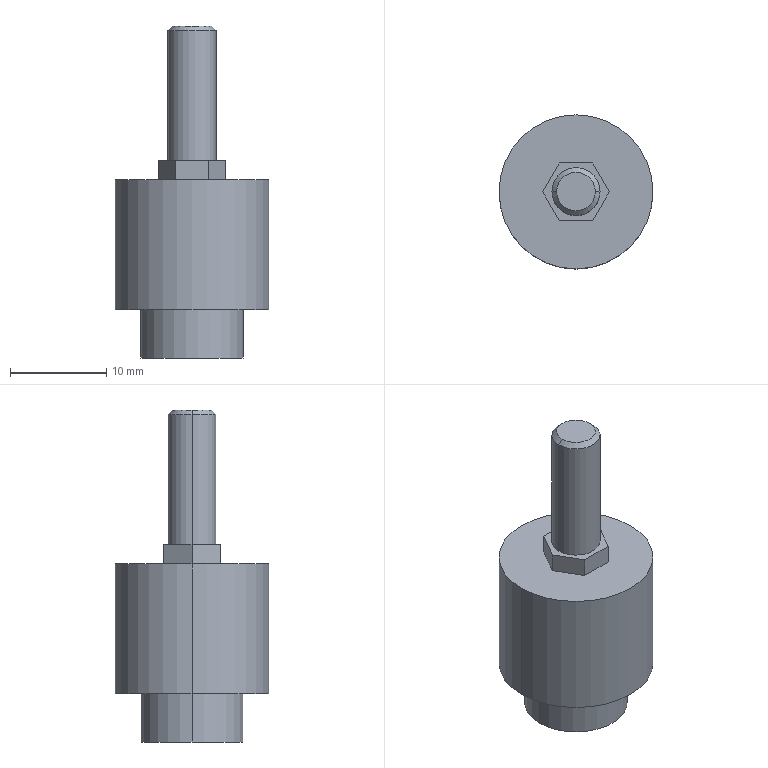Part | STEP file | JA15_5_080 | 1 solid | 24 faces | box 16 x 16 x 34.5 mm | volume 3402 mm3 | plane 12 | cylinder 8 | cone 4 | commonest cylinder face diameters 4.13 x2 5 x2 10.667 x2 16 x2
STEP:
#1=CARTESIAN_POINT('',(0.,0.,0.));
#2=DIRECTION('',(0.,0.,1.));
#3=DIRECTION('',(1.,0.,0.));
#4=AXIS2_PLACEMENT_3D('',#1,#2,#3);
#5=CARTESIAN_POINT('',(-2.5,0.,34.01));
#6=VERTEX_POINT('',#5);
#7=CARTESIAN_POINT('',(2.5,0.,34.01));
#8=VERTEX_POINT('',#7);
#9=CARTESIAN_POINT('',(0.,0.,34.01));
#10=DIRECTION('',(0.,0.,-1.));
#11=DIRECTION('',(-1.,0.,0.));
#12=AXIS2_PLACEMENT_3D('',#9,#10,#11);
#13=CIRCLE('',#12,2.5);
#14=CARTESIAN_POINT('',(0.,0.,20.5));
#15=DIRECTION('',(0.,0.,-1.));
#16=DIRECTION('',(-1.,0.,0.));
#17=AXIS2_PLACEMENT_3D('',#14,#15,#16);
#18=CYLINDRICAL_SURFACE('',#17,2.5);
#19=CARTESIAN_POINT('',(0.,-13.51));
#20=DIRECTION('',(1.,0.));
#21=VECTOR('',#20,1.);
#22=LINE('',#19,#21);
#23=(GEOMETRIC_REPRESENTATION_CONTEXT(2)PARAMETRIC_REPRESENTATION_CONTEXT()REPRESENTATION_CONTEXT('',''));
#24=DEFINITIONAL_REPRESENTATION('',(#22),#23);
#25=PCURVE('',#18,#24);
#26=CARTESIAN_POINT('',(0.,0.,34.01));
#27=DIRECTION('',(0.,0.,-1.));
#28=DIRECTION('',(-1.,0.,0.));
#29=AXIS2_PLACEMENT_3D('',#26,#27,#28);
#30=CONICAL_SURFACE('',#29,2.5,0.7854);
#31=CARTESIAN_POINT('',(0.,0.));
#32=DIRECTION('',(1.,0.));
#33=VECTOR('',#32,1.);
#34=LINE('',#31,#33);
#35=(GEOMETRIC_REPRESENTATION_CONTEXT(2)PARAMETRIC_REPRESENTATION_CONTEXT()REPRESENTATION_CONTEXT('',''));
#36=DEFINITIONAL_REPRESENTATION('',(#34),#35);
#37=PCURVE('',#30,#36);
#38=SURFACE_CURVE('',#13,(#25,#37),.PCURVE_S1.);
#39=EDGE_CURVE('',#6,#8,#38,.T.);
#40=ORIENTED_EDGE('',*,*,#39,.T.);
#41=CARTESIAN_POINT('',(2.5,0.,20.5));
#42=VERTEX_POINT('',#41);
#43=CARTESIAN_POINT('',(2.5,0.,20.5));
#44=DIRECTION('',(0.,0.,-1.));
#45=VECTOR('',#44,1.);
#46=LINE('',#43,#45);
#47=CARTESIAN_POINT('',(3.142,0.));
#48=DIRECTION('',(0.,1.));
#49=VECTOR('',#48,1.);
#50=LINE('',#47,#49);
#51=(GEOMETRIC_REPRESENTATION_CONTEXT(2)PARAMETRIC_REPRESENTATION_CONTEXT()REPRESENTATION_CONTEXT('',''));
#52=DEFINITIONAL_REPRESENTATION('',(#50),#51);
#53=PCURVE('',#18,#52);
#54=CARTESIAN_POINT('',(0.,0.,20.5));
#55=DIRECTION('',(0.,0.,-1.));
#56=DIRECTION('',(-1.,0.,0.));
#57=AXIS2_PLACEMENT_3D('',#54,#55,#56);
#58=CYLINDRICAL_SURFACE('',#57,2.5);
#59=CARTESIAN_POINT('',(3.142,0.));
#60=DIRECTION('',(0.,1.));
#61=VECTOR('',#60,1.);
#62=LINE('',#59,#61);
#63=(GEOMETRIC_REPRESENTATION_CONTEXT(2)PARAMETRIC_REPRESENTATION_CONTEXT()REPRESENTATION_CONTEXT('',''));
#64=DEFINITIONAL_REPRESENTATION('',(#62),#63);
#65=PCURVE('',#58,#64);
#66=SURFACE_CURVE('',#46,(#53,#65),.PCURVE_S1.);
#67=EDGE_CURVE('',#8,#42,#66,.T.);
#68=ORIENTED_EDGE('',*,*,#67,.T.);
#69=CARTESIAN_POINT('',(-2.5,0.,20.5));
#70=VERTEX_POINT('',#69);
#71=CARTESIAN_POINT('',(0.,0.,20.5));
#72=DIRECTION('',(0.,0.,1.));
#73=DIRECTION('',(1.,0.,0.));
#74=AXIS2_PLACEMENT_3D('',#71,#72,#73);
#75=CIRCLE('',#74,2.5);
#76=CARTESIAN_POINT('',(3.142,0.));
#77=DIRECTION('',(-1.,0.));
#78=VECTOR('',#77,1.);
#79=LINE('',#76,#78);
#80=(GEOMETRIC_REPRESENTATION_CONTEXT(2)PARAMETRIC_REPRESENTATION_CONTEXT()REPRESENTATION_CONTEXT('',''));
#81=DEFINITIONAL_REPRESENTATION('',(#79),#80);
#82=PCURVE('',#18,#81);
#83=CARTESIAN_POINT('',(-1.732,-3.,20.5));
#84=DIRECTION('',(0.,0.,1.));
#85=DIRECTION('',(1.,0.,0.));
#86=AXIS2_PLACEMENT_3D('',#83,#84,#85);
#87=PLANE('',#86);
#88=CARTESIAN_POINT('',(1.732,3.));
#89=DIRECTION('',(1.,0.));
#90=AXIS2_PLACEMENT_2D('',#88,#89);
#91=CIRCLE('',#90,2.5);
#92=(GEOMETRIC_REPRESENTATION_CONTEXT(2)PARAMETRIC_REPRESENTATION_CONTEXT()REPRESENTATION_CONTEXT('',''));
#93=DEFINITIONAL_REPRESENTATION('',(#91),#92);
#94=PCURVE('',#87,#93);
#95=SURFACE_CURVE('',#75,(#82,#94),.PCURVE_S1.);
#96=EDGE_CURVE('',#42,#70,#95,.T.);
#97=ORIENTED_EDGE('',*,*,#96,.T.);
#98=CARTESIAN_POINT('',(-2.5,0.,20.5));
#99=DIRECTION('',(0.,0.,-1.));
#100=VECTOR('',#99,1.);
#101=LINE('',#98,#100);
#102=CARTESIAN_POINT('',(0.,0.));
#103=DIRECTION('',(0.,1.));
#104=VECTOR('',#103,1.);
#105=LINE('',#102,#104);
#106=(GEOMETRIC_REPRESENTATION_CONTEXT(2)PARAMETRIC_REPRESENTATION_CONTEXT()REPRESENTATION_CONTEXT('',''));
#107=DEFINITIONAL_REPRESENTATION('',(#105),#106);
#108=PCURVE('',#18,#107);
#109=CARTESIAN_POINT('',(6.283,0.));
#110=DIRECTION('',(0.,1.));
#111=VECTOR('',#110,1.);
#112=LINE('',#109,#111);
#113=(GEOMETRIC_REPRESENTATION_CONTEXT(2)PARAMETRIC_REPRESENTATION_CONTEXT()REPRESENTATION_CONTEXT('',''));
#114=DEFINITIONAL_REPRESENTATION('',(#112),#113);
#115=PCURVE('',#58,#114);
#116=SURFACE_CURVE('',#101,(#108,#115),.PCURVE_S1.);
#117=EDGE_CURVE('',#6,#70,#116,.T.);
#118=ORIENTED_EDGE('',*,*,#117,.F.);
#119=EDGE_LOOP('',(#40,#68,#97,#118));
#120=FACE_BOUND('',#119,.T.);
#121=ADVANCED_FACE('',(#120),#18,.T.);
#122=CARTESIAN_POINT('',(-2.01,0.,34.5));
#123=VERTEX_POINT('',#122);
#124=CARTESIAN_POINT('',(2.01,0.,34.5));
#125=VERTEX_POINT('',#124);
#126=CARTESIAN_POINT('',(0.,0.,34.5));
#127=DIRECTION('',(0.,0.,-1.));
#128=DIRECTION('',(-1.,0.,0.));
#129=AXIS2_PLACEMENT_3D('',#126,#127,#128);
#130=CIRCLE('',#129,2.01);
#131=CARTESIAN_POINT('',(0.,-0.49));
#132=DIRECTION('',(1.,0.));
#133=VECTOR('',#132,1.);
#134=LINE('',#131,#133);
#135=(GEOMETRIC_REPRESENTATION_CONTEXT(2)PARAMETRIC_REPRESENTATION_CONTEXT()REPRESENTATION_CONTEXT('',''));
#136=DEFINITIONAL_REPRESENTATION('',(#134),#135);
#137=PCURVE('',#30,#136);
#138=CARTESIAN_POINT('',(0.,0.,34.5));
#139=DIRECTION('',(0.,0.,1.));
#140=DIRECTION('',(1.,0.,0.));
#141=AXIS2_PLACEMENT_3D('',#138,#139,#140);
#142=PLANE('',#141);
#143=CARTESIAN_POINT('',(-2.01,0.));
#144=CARTESIAN_POINT('',(-2.01,3.481));
#145=CARTESIAN_POINT('',(1.005,1.741));
#146=CARTESIAN_POINT('',(4.02,0.));
#147=CARTESIAN_POINT('',(1.005,-1.741));
#148=CARTESIAN_POINT('',(-2.01,-3.481));
#149=CARTESIAN_POINT('',(-2.01,0.));
#150=(BOUNDED_CURVE()B_SPLINE_CURVE(2,(#143,#144,#145,#146,#147,#148,#149),.UNSPECIFIED.,.T.,.F.)B_SPLINE_CURVE_WITH_KNOTS((1,2,2,2,2,1),(-2.094,0.,2.094,4.189,6.283,8.378),.UNSPECIFIED.)CURVE()GEOMETRIC_REPRESENTATION_ITEM()RATIONAL_B_SPLINE_CURVE((1.,0.5,1.,0.5,1.,0.5,1.))REPRESENTATION_ITEM(''));
#151=(GEOMETRIC_REPRESENTATION_CONTEXT(2)PARAMETRIC_REPRESENTATION_CONTEXT()REPRESENTATION_CONTEXT('',''));
#152=DEFINITIONAL_REPRESENTATION('',(#150),#151);
#153=PCURVE('',#142,#152);
#154=SURFACE_CURVE('',#130,(#137,#153),.PCURVE_S1.);
#155=EDGE_CURVE('',#123,#125,#154,.T.);
#156=ORIENTED_EDGE('',*,*,#155,.T.);
#157=CARTESIAN_POINT('',(2.5,0.,34.01));
#158=DIRECTION('',(0.7071,0.,-0.7071));
#159=VECTOR('',#158,1.);
#160=LINE('',#157,#159);
#161=CARTESIAN_POINT('',(3.142,0.));
#162=DIRECTION('',(0.,1.));
#163=VECTOR('',#162,1.);
#164=LINE('',#161,#163);
#165=(GEOMETRIC_REPRESENTATION_CONTEXT(2)PARAMETRIC_REPRESENTATION_CONTEXT()REPRESENTATION_CONTEXT('',''));
#166=DEFINITIONAL_REPRESENTATION('',(#164),#165);
#167=PCURVE('',#30,#166);
#168=CARTESIAN_POINT('',(0.,0.,34.01));
#169=DIRECTION('',(0.,0.,-1.));
#170=DIRECTION('',(-1.,0.,0.));
#171=AXIS2_PLACEMENT_3D('',#168,#169,#170);
#172=CONICAL_SURFACE('',#171,2.5,0.7854);
#173=CARTESIAN_POINT('',(3.142,0.));
#174=DIRECTION('',(0.,1.));
#175=VECTOR('',#174,1.);
#176=LINE('',#173,#175);
#177=(GEOMETRIC_REPRESENTATION_CONTEXT(2)PARAMETRIC_REPRESENTATION_CONTEXT()REPRESENTATION_CONTEXT('',''));
#178=DEFINITIONAL_REPRESENTATION('',(#176),#177);
#179=PCURVE('',#172,#178);
#180=SURFACE_CURVE('',#160,(#167,#179),.PCURVE_S1.);
#181=EDGE_CURVE('',#125,#8,#180,.T.);
#182=ORIENTED_EDGE('',*,*,#181,.T.);
#183=ORIENTED_EDGE('',*,*,#39,.F.);
#184=CARTESIAN_POINT('',(-2.5,0.,34.01));
#185=DIRECTION('',(-0.7071,0.,-0.7071));
#186=VECTOR('',#185,1.);
#187=LINE('',#184,#186);
#188=CARTESIAN_POINT('',(0.,0.));
#189=DIRECTION('',(0.,1.));
#190=VECTOR('',#189,1.);
#191=LINE('',#188,#190);
#192=(GEOMETRIC_REPRESENTATION_CONTEXT(2)PARAMETRIC_REPRESENTATION_CONTEXT()REPRESENTATION_CONTEXT('',''));
#193=DEFINITIONAL_REPRESENTATION('',(#191),#192);
#194=PCURVE('',#30,#193);
#195=CARTESIAN_POINT('',(6.283,0.));
#196=DIRECTION('',(0.,1.));
#197=VECTOR('',#196,1.);
#198=LINE('',#195,#197);
#199=(GEOMETRIC_REPRESENTATION_CONTEXT(2)PARAMETRIC_REPRESENTATION_CONTEXT()REPRESENTATION_CONTEXT('',''));
#200=DEFINITIONAL_REPRESENTATION('',(#198),#199);
#201=PCURVE('',#172,#200);
#202=SURFACE_CURVE('',#187,(#194,#201),.PCURVE_S1.);
#203=EDGE_CURVE('',#123,#6,#202,.T.);
#204=ORIENTED_EDGE('',*,*,#203,.F.);
#205=EDGE_LOOP('',(#156,#182,#183,#204));
#206=FACE_BOUND('',#205,.T.);
#207=ADVANCED_FACE('',(#206),#30,.T.);
#208=CARTESIAN_POINT('',(-2.065,0.,7.));
#209=VERTEX_POINT('',#208);
#210=CARTESIAN_POINT('',(-2.065,0.,0.435));
#211=VERTEX_POINT('',#210);
#212=CARTESIAN_POINT('',(-2.065,0.,0.));
#213=DIRECTION('',(0.,0.,-1.));
#214=VECTOR('',#213,1.);
#215=LINE('',#212,#214);
#216=CARTESIAN_POINT('',(0.,0.,0.));
#217=DIRECTION('',(0.,0.,-1.));
#218=DIRECTION('',(-1.,0.,0.));
#219=AXIS2_PLACEMENT_3D('',#216,#217,#218);
#220=CYLINDRICAL_SURFACE('',#219,2.065);
#221=CARTESIAN_POINT('',(6.283,0.));
#222=DIRECTION('',(0.,1.));
#223=VECTOR('',#222,1.);
#224=LINE('',#221,#223);
#225=(GEOMETRIC_REPRESENTATION_CONTEXT(2)PARAMETRIC_REPRESENTATION_CONTEXT()REPRESENTATION_CONTEXT('',''));
#226=DEFINITIONAL_REPRESENTATION('',(#224),#225);
#227=PCURVE('',#220,#226);
#228=CARTESIAN_POINT('',(0.,0.,0.));
#229=DIRECTION('',(0.,0.,-1.));
#230=DIRECTION('',(-1.,0.,0.));
#231=AXIS2_PLACEMENT_3D('',#228,#229,#230);
#232=CYLINDRICAL_SURFACE('',#231,2.065);
#233=CARTESIAN_POINT('',(0.,0.));
#234=DIRECTION('',(0.,1.));
#235=VECTOR('',#234,1.);
#236=LINE('',#233,#235);
#237=(GEOMETRIC_REPRESENTATION_CONTEXT(2)PARAMETRIC_REPRESENTATION_CONTEXT()REPRESENTATION_CONTEXT('',''));
#238=DEFINITIONAL_REPRESENTATION('',(#236),#237);
#239=PCURVE('',#232,#238);
#240=SURFACE_CURVE('',#215,(#227,#239),.PCURVE_S1.);
#241=EDGE_CURVE('',#209,#211,#240,.T.);
#242=ORIENTED_EDGE('',*,*,#241,.T.);
#243=CARTESIAN_POINT('',(2.065,0.,0.435));
#244=VERTEX_POINT('',#243);
#245=CARTESIAN_POINT('',(0.,0.,0.435));
#246=DIRECTION('',(0.,0.,-1.));
#247=DIRECTION('',(-1.,0.,0.));
#248=AXIS2_PLACEMENT_3D('',#245,#246,#247);
#249=CIRCLE('',#248,2.065);
#250=CARTESIAN_POINT('',(0.,-0.435));
#251=DIRECTION('',(1.,0.));
#252=VECTOR('',#251,1.);
#253=LINE('',#250,#252);
#254=(GEOMETRIC_REPRESENTATION_CONTEXT(2)PARAMETRIC_REPRESENTATION_CONTEXT()REPRESENTATION_CONTEXT('',''));
#255=DEFINITIONAL_REPRESENTATION('',(#253),#254);
#256=PCURVE('',#220,#255);
#257=CARTESIAN_POINT('',(0.,0.,0.435));
#258=DIRECTION('',(0.,0.,-1.));
#259=DIRECTION('',(-1.,0.,0.));
#260=AXIS2_PLACEMENT_3D('',#257,#258,#259);
#261=CONICAL_SURFACE('',#260,2.065,0.7854);
#262=CARTESIAN_POINT('',(0.,0.));
#263=DIRECTION('',(1.,0.));
#264=VECTOR('',#263,1.);
#265=LINE('',#262,#264);
#266=(GEOMETRIC_REPRESENTATION_CONTEXT(2)PARAMETRIC_REPRESENTATION_CONTEXT()REPRESENTATION_CONTEXT('',''));
#267=DEFINITIONAL_REPRESENTATION('',(#265),#266);
#268=PCURVE('',#261,#267);
#269=SURFACE_CURVE('',#249,(#256,#268),.PCURVE_S1.);
#270=EDGE_CURVE('',#244,#211,#269,.T.);
#271=ORIENTED_EDGE('',*,*,#270,.F.);
#272=CARTESIAN_POINT('',(2.065,0.,7.));
#273=VERTEX_POINT('',#272);
#274=CARTESIAN_POINT('',(2.065,0.,0.));
#275=DIRECTION('',(0.,0.,-1.));
#276=VECTOR('',#275,1.);
#277=LINE('',#274,#276);
#278=CARTESIAN_POINT('',(3.142,0.));
#279=DIRECTION('',(0.,1.));
#280=VECTOR('',#279,1.);
#281=LINE('',#278,#280);
#282=(GEOMETRIC_REPRESENTATION_CONTEXT(2)PARAMETRIC_REPRESENTATION_CONTEXT()REPRESENTATION_CONTEXT('',''));
#283=DEFINITIONAL_REPRESENTATION('',(#281),#282);
#284=PCURVE('',#220,#283);
#285=CARTESIAN_POINT('',(3.142,0.));
#286=DIRECTION('',(0.,1.));
#287=VECTOR('',#286,1.);
#288=LINE('',#285,#287);
#289=(GEOMETRIC_REPRESENTATION_CONTEXT(2)PARAMETRIC_REPRESENTATION_CONTEXT()REPRESENTATION_CONTEXT('',''));
#290=DEFINITIONAL_REPRESENTATION('',(#288),#289);
#291=PCURVE('',#232,#290);
#292=SURFACE_CURVE('',#277,(#284,#291),.PCURVE_S1.);
#293=EDGE_CURVE('',#273,#244,#292,.T.);
#294=ORIENTED_EDGE('',*,*,#293,.F.);
#295=CARTESIAN_POINT('',(0.,0.,7.));
#296=DIRECTION('',(0.,0.,-1.));
#297=DIRECTION('',(-1.,0.,0.));
#298=AXIS2_PLACEMENT_3D('',#295,#296,#297);
#299=CIRCLE('',#298,2.065);
#300=CARTESIAN_POINT('',(0.,-7.));
#301=DIRECTION('',(1.,0.));
#302=VECTOR('',#301,1.);
#303=LINE('',#300,#302);
#304=(GEOMETRIC_REPRESENTATION_CONTEXT(2)PARAMETRIC_REPRESENTATION_CONTEXT()REPRESENTATION_CONTEXT('',''));
#305=DEFINITIONAL_REPRESENTATION('',(#303),#304);
#306=PCURVE('',#220,#305);
#307=CARTESIAN_POINT('',(0.,2.065,7.));
#308=DIRECTION('',(0.,0.,-1.));
#309=DIRECTION('',(-1.,0.,0.));
#310=AXIS2_PLACEMENT_3D('',#307,#308,#309);
#311=PLANE('',#310);
#312=CARTESIAN_POINT('',(0.,-2.065));
#313=DIRECTION('',(1.,0.));
#314=AXIS2_PLACEMENT_2D('',#312,#313);
#315=CIRCLE('',#314,2.065);
#316=(GEOMETRIC_REPRESENTATION_CONTEXT(2)PARAMETRIC_REPRESENTATION_CONTEXT()REPRESENTATION_CONTEXT('',''));
#317=DEFINITIONAL_REPRESENTATION('',(#315),#316);
#318=PCURVE('',#311,#317);
#319=SURFACE_CURVE('',#299,(#306,#318),.PCURVE_S1.);
#320=EDGE_CURVE('',#273,#209,#319,.T.);
#321=ORIENTED_EDGE('',*,*,#320,.T.);
#322=EDGE_LOOP('',(#242,#271,#294,#321));
#323=FACE_BOUND('',#322,.F.);
#324=ADVANCED_FACE('',(#323),#220,.F.);
#325=CARTESIAN_POINT('',(-2.5,0.,0.));
#326=VERTEX_POINT('',#325);
#327=CARTESIAN_POINT('',(-2.065,0.,0.435));
#328=DIRECTION('',(-0.7071,0.,-0.7071));
#329=VECTOR('',#328,1.);
#330=LINE('',#327,#329);
#331=CARTESIAN_POINT('',(6.283,0.));
#332=DIRECTION('',(0.,1.));
#333=VECTOR('',#332,1.);
#334=LINE('',#331,#333);
#335=(GEOMETRIC_REPRESENTATION_CONTEXT(2)PARAMETRIC_REPRESENTATION_CONTEXT()REPRESENTATION_CONTEXT('',''));
#336=DEFINITIONAL_REPRESENTATION('',(#334),#335);
#337=PCURVE('',#261,#336);
#338=CARTESIAN_POINT('',(0.,0.,0.435));
#339=DIRECTION('',(0.,0.,-1.));
#340=DIRECTION('',(-1.,0.,0.));
#341=AXIS2_PLACEMENT_3D('',#338,#339,#340);
#342=CONICAL_SURFACE('',#341,2.065,0.7854);
#343=CARTESIAN_POINT('',(0.,0.));
#344=DIRECTION('',(0.,1.));
#345=VECTOR('',#344,1.);
#346=LINE('',#343,#345);
#347=(GEOMETRIC_REPRESENTATION_CONTEXT(2)PARAMETRIC_REPRESENTATION_CONTEXT()REPRESENTATION_CONTEXT('',''));
#348=DEFINITIONAL_REPRESENTATION('',(#346),#347);
#349=PCURVE('',#342,#348);
#350=SURFACE_CURVE('',#330,(#337,#349),.PCURVE_S1.);
#351=EDGE_CURVE('',#211,#326,#350,.T.);
#352=ORIENTED_EDGE('',*,*,#351,.T.);
#353=CARTESIAN_POINT('',(2.5,0.,0.));
#354=VERTEX_POINT('',#353);
#355=CARTESIAN_POINT('',(0.,0.,0.));
#356=DIRECTION('',(0.,0.,-1.));
#357=DIRECTION('',(-1.,0.,0.));
#358=AXIS2_PLACEMENT_3D('',#355,#356,#357);
#359=CIRCLE('',#358,2.5);
#360=CARTESIAN_POINT('',(0.,0.435));
#361=DIRECTION('',(1.,0.));
#362=VECTOR('',#361,1.);
#363=LINE('',#360,#362);
#364=(GEOMETRIC_REPRESENTATION_CONTEXT(2)PARAMETRIC_REPRESENTATION_CONTEXT()REPRESENTATION_CONTEXT('',''));
#365=DEFINITIONAL_REPRESENTATION('',(#363),#364);
#366=PCURVE('',#261,#365);
#367=CARTESIAN_POINT('',(0.,5.333,0.));
#368=DIRECTION('',(0.,0.,-1.));
#369=DIRECTION('',(-1.,0.,0.));
#370=AXIS2_PLACEMENT_3D('',#367,#368,#369);
#371=PLANE('',#370);
#372=CARTESIAN_POINT('',(0.,-5.333));
#373=DIRECTION('',(1.,0.));
#374=AXIS2_PLACEMENT_2D('',#372,#373);
#375=CIRCLE('',#374,2.5);
#376=(GEOMETRIC_REPRESENTATION_CONTEXT(2)PARAMETRIC_REPRESENTATION_CONTEXT()REPRESENTATION_CONTEXT('',''));
#377=DEFINITIONAL_REPRESENTATION('',(#375),#376);
#378=PCURVE('',#371,#377);
#379=SURFACE_CURVE('',#359,(#366,#378),.PCURVE_S1.);
#380=EDGE_CURVE('',#354,#326,#379,.T.);
#381=ORIENTED_EDGE('',*,*,#380,.F.);
#382=CARTESIAN_POINT('',(2.065,0.,0.435));
#383=DIRECTION('',(0.7071,0.,-0.7071));
#384=VECTOR('',#383,1.);
#385=LINE('',#382,#384);
#386=CARTESIAN_POINT('',(3.142,0.));
#387=DIRECTION('',(0.,1.));
#388=VECTOR('',#387,1.);
#389=LINE('',#386,#388);
#390=(GEOMETRIC_REPRESENTATION_CONTEXT(2)PARAMETRIC_REPRESENTATION_CONTEXT()REPRESENTATION_CONTEXT('',''));
#391=DEFINITIONAL_REPRESENTATION('',(#389),#390);
#392=PCURVE('',#261,#391);
#393=CARTESIAN_POINT('',(3.142,0.));
#394=DIRECTION('',(0.,1.));
#395=VECTOR('',#394,1.);
#396=LINE('',#393,#395);
#397=(GEOMETRIC_REPRESENTATION_CONTEXT(2)PARAMETRIC_REPRESENTATION_CONTEXT()REPRESENTATION_CONTEXT('',''));
#398=DEFINITIONAL_REPRESENTATION('',(#396),#397);
#399=PCURVE('',#342,#398);
#400=SURFACE_CURVE('',#385,(#392,#399),.PCURVE_S1.);
#401=EDGE_CURVE('',#244,#354,#400,.T.);
#402=ORIENTED_EDGE('',*,*,#401,.F.);
#403=ORIENTED_EDGE('',*,*,#270,.T.);
#404=EDGE_LOOP('',(#352,#381,#402,#403));
#405=FACE_BOUND('',#404,.F.);
#406=ADVANCED_FACE('',(#405),#261,.F.);
#407=CARTESIAN_POINT('',(-5.333,0.,5.));
#408=VERTEX_POINT('',#407);
#409=CARTESIAN_POINT('',(5.333,0.,5.));
#410=VERTEX_POINT('',#409);
#411=CARTESIAN_POINT('',(0.,0.,5.));
#412=DIRECTION('',(0.,0.,-1.));
#413=DIRECTION('',(-1.,0.,0.));
#414=AXIS2_PLACEMENT_3D('',#411,#412,#413);
#415=CIRCLE('',#414,5.333);
#416=CARTESIAN_POINT('',(0.,0.,0.));
#417=DIRECTION('',(0.,0.,-1.));
#418=DIRECTION('',(-1.,0.,0.));
#419=AXIS2_PLACEMENT_3D('',#416,#417,#418);
#420=CYLINDRICAL_SURFACE('',#419,5.333);
#421=CARTESIAN_POINT('',(0.,-5.));
#422=DIRECTION('',(1.,0.));
#423=VECTOR('',#422,1.);
#424=LINE('',#421,#423);
#425=(GEOMETRIC_REPRESENTATION_CONTEXT(2)PARAMETRIC_REPRESENTATION_CONTEXT()REPRESENTATION_CONTEXT('',''));
#426=DEFINITIONAL_REPRESENTATION('',(#424),#425);
#427=PCURVE('',#420,#426);
#428=CARTESIAN_POINT('',(0.,8.,5.));
#429=DIRECTION('',(0.,0.,-1.));
#430=DIRECTION('',(-1.,0.,0.));
#431=AXIS2_PLACEMENT_3D('',#428,#429,#430);
#432=PLANE('',#431);
#433=CARTESIAN_POINT('',(0.,-8.));
#434=DIRECTION('',(1.,0.));
#435=AXIS2_PLACEMENT_2D('',#433,#434);
#436=CIRCLE('',#435,5.333);
#437=(GEOMETRIC_REPRESENTATION_CONTEXT(2)PARAMETRIC_REPRESENTATION_CONTEXT()REPRESENTATION_CONTEXT('',''));
#438=DEFINITIONAL_REPRESENTATION('',(#436),#437);
#439=PCURVE('',#432,#438);
#440=SURFACE_CURVE('',#415,(#427,#439),.PCURVE_S1.);
#441=EDGE_CURVE('',#408,#410,#440,.T.);
#442=ORIENTED_EDGE('',*,*,#441,.T.);
#443=CARTESIAN_POINT('',(5.333,0.,0.));
#444=VERTEX_POINT('',#443);
#445=CARTESIAN_POINT('',(5.333,0.,0.));
#446=DIRECTION('',(0.,0.,-1.));
#447=VECTOR('',#446,1.);
#448=LINE('',#445,#447);
#449=CARTESIAN_POINT('',(3.142,0.));
#450=DIRECTION('',(0.,1.));
#451=VECTOR('',#450,1.);
#452=LINE('',#449,#451);
#453=(GEOMETRIC_REPRESENTATION_CONTEXT(2)PARAMETRIC_REPRESENTATION_CONTEXT()REPRESENTATION_CONTEXT('',''));
#454=DEFINITIONAL_REPRESENTATION('',(#452),#453);
#455=PCURVE('',#420,#454);
#456=CARTESIAN_POINT('',(0.,0.,0.));
#457=DIRECTION('',(0.,0.,-1.));
#458=DIRECTION('',(-1.,0.,0.));
#459=AXIS2_PLACEMENT_3D('',#456,#457,#458);
#460=CYLINDRICAL_SURFACE('',#459,5.333);
#461=CARTESIAN_POINT('',(3.142,0.));
#462=DIRECTION('',(0.,1.));
#463=VECTOR('',#462,1.);
#464=LINE('',#461,#463);
#465=(GEOMETRIC_REPRESENTATION_CONTEXT(2)PARAMETRIC_REPRESENTATION_CONTEXT()REPRESENTATION_CONTEXT('',''));
#466=DEFINITIONAL_REPRESENTATION('',(#464),#465);
#467=PCURVE('',#460,#466);
#468=SURFACE_CURVE('',#448,(#455,#467),.PCURVE_S1.);
#469=EDGE_CURVE('',#410,#444,#468,.T.);
#470=ORIENTED_EDGE('',*,*,#469,.T.);
#471=CARTESIAN_POINT('',(-5.333,0.,0.));
#472=VERTEX_POINT('',#471);
#473=CARTESIAN_POINT('',(0.,0.,0.));
#474=DIRECTION('',(0.,0.,-1.));
#475=DIRECTION('',(-1.,0.,0.));
#476=AXIS2_PLACEMENT_3D('',#473,#474,#475);
#477=CIRCLE('',#476,5.333);
#478=CARTESIAN_POINT('',(0.,0.));
#479=DIRECTION('',(1.,0.));
#480=VECTOR('',#479,1.);
#481=LINE('',#478,#480);
#482=(GEOMETRIC_REPRESENTATION_CONTEXT(2)PARAMETRIC_REPRESENTATION_CONTEXT()REPRESENTATION_CONTEXT('',''));
#483=DEFINITIONAL_REPRESENTATION('',(#481),#482);
#484=PCURVE('',#420,#483);
#485=CARTESIAN_POINT('',(0.,-5.333));
#486=DIRECTION('',(1.,0.));
#487=AXIS2_PLACEMENT_2D('',#485,#486);
#488=CIRCLE('',#487,5.333);
#489=(GEOMETRIC_REPRESENTATION_CONTEXT(2)PARAMETRIC_REPRESENTATION_CONTEXT()REPRESENTATION_CONTEXT('',''));
#490=DEFINITIONAL_REPRESENTATION('',(#488),#489);
#491=PCURVE('',#371,#490);
#492=SURFACE_CURVE('',#477,(#484,#491),.PCURVE_S1.);
#493=EDGE_CURVE('',#472,#444,#492,.T.);
#494=ORIENTED_EDGE('',*,*,#493,.F.);
#495=CARTESIAN_POINT('',(-5.333,0.,0.));
#496=DIRECTION('',(0.,0.,-1.));
#497=VECTOR('',#496,1.);
#498=LINE('',#495,#497);
#499=CARTESIAN_POINT('',(0.,0.));
#500=DIRECTION('',(0.,1.));
#501=VECTOR('',#500,1.);
#502=LINE('',#499,#501);
#503=(GEOMETRIC_REPRESENTATION_CONTEXT(2)PARAMETRIC_REPRESENTATION_CONTEXT()REPRESENTATION_CONTEXT('',''));
#504=DEFINITIONAL_REPRESENTATION('',(#502),#503);
#505=PCURVE('',#420,#504);
#506=CARTESIAN_POINT('',(6.283,0.));
#507=DIRECTION('',(0.,1.));
#508=VECTOR('',#507,1.);
#509=LINE('',#506,#508);
#510=(GEOMETRIC_REPRESENTATION_CONTEXT(2)PARAMETRIC_REPRESENTATION_CONTEXT()REPRESENTATION_CONTEXT('',''));
#511=DEFINITIONAL_REPRESENTATION('',(#509),#510);
#512=PCURVE('',#460,#511);
#513=SURFACE_CURVE('',#498,(#505,#512),.PCURVE_S1.);
#514=EDGE_CURVE('',#408,#472,#513,.T.);
#515=ORIENTED_EDGE('',*,*,#514,.F.);
#516=EDGE_LOOP('',(#442,#470,#494,#515));
#517=FACE_BOUND('',#516,.T.);
#518=ADVANCED_FACE('',(#517),#420,.T.);
#519=CARTESIAN_POINT('',(-8.,0.,18.5));
#520=VERTEX_POINT('',#519);
#521=CARTESIAN_POINT('',(8.,0.,18.5));
#522=VERTEX_POINT('',#521);
#523=CARTESIAN_POINT('',(0.,0.,18.5));
#524=DIRECTION('',(0.,0.,-1.));
#525=DIRECTION('',(-1.,0.,0.));
#526=AXIS2_PLACEMENT_3D('',#523,#524,#525);
#527=CIRCLE('',#526,8.);
#528=CARTESIAN_POINT('',(0.,0.,0.));
#529=DIRECTION('',(0.,0.,-1.));
#530=DIRECTION('',(-1.,0.,0.));
#531=AXIS2_PLACEMENT_3D('',#528,#529,#530);
#532=CYLINDRICAL_SURFACE('',#531,8.);
#533=CARTESIAN_POINT('',(0.,-18.5));
#534=DIRECTION('',(1.,0.));
#535=VECTOR('',#534,1.);
#536=LINE('',#533,#535);
#537=(GEOMETRIC_REPRESENTATION_CONTEXT(2)PARAMETRIC_REPRESENTATION_CONTEXT()REPRESENTATION_CONTEXT('',''));
#538=DEFINITIONAL_REPRESENTATION('',(#536),#537);
#539=PCURVE('',#532,#538);
#540=CARTESIAN_POINT('',(0.,0.,18.5));
#541=DIRECTION('',(0.,0.,1.));
#542=DIRECTION('',(1.,0.,0.));
#543=AXIS2_PLACEMENT_3D('',#540,#541,#542);
#544=PLANE('',#543);
#545=CARTESIAN_POINT('',(-8.,0.));
#546=CARTESIAN_POINT('',(-8.,13.856));
#547=CARTESIAN_POINT('',(4.,6.928));
#548=CARTESIAN_POINT('',(16.,0.));
#549=CARTESIAN_POINT('',(4.,-6.928));
#550=CARTESIAN_POINT('',(-8.,-13.856));
#551=CARTESIAN_POINT('',(-8.,0.));
#552=(BOUNDED_CURVE()B_SPLINE_CURVE(2,(#545,#546,#547,#548,#549,#550,#551),.UNSPECIFIED.,.T.,.F.)B_SPLINE_CURVE_WITH_KNOTS((1,2,2,2,2,1),(-2.094,0.,2.094,4.189,6.283,8.378),.UNSPECIFIED.)CURVE()GEOMETRIC_REPRESENTATION_ITEM()RATIONAL_B_SPLINE_CURVE((1.,0.5,1.,0.5,1.,0.5,1.))REPRESENTATION_ITEM(''));
#553=(GEOMETRIC_REPRESENTATION_CONTEXT(2)PARAMETRIC_REPRESENTATION_CONTEXT()REPRESENTATION_CONTEXT('',''));
#554=DEFINITIONAL_REPRESENTATION('',(#552),#553);
#555=PCURVE('',#544,#554);
#556=SURFACE_CURVE('',#527,(#539,#555),.PCURVE_S1.);
#557=EDGE_CURVE('',#520,#522,#556,.T.);
#558=ORIENTED_EDGE('',*,*,#557,.T.);
#559=CARTESIAN_POINT('',(8.,0.,5.));
#560=VERTEX_POINT('',#559);
#561=CARTESIAN_POINT('',(8.,0.,0.));
#562=DIRECTION('',(0.,0.,-1.));
#563=VECTOR('',#562,1.);
#564=LINE('',#561,#563);
#565=CARTESIAN_POINT('',(3.142,0.));
#566=DIRECTION('',(0.,1.));
#567=VECTOR('',#566,1.);
#568=LINE('',#565,#567);
#569=(GEOMETRIC_REPRESENTATION_CONTEXT(2)PARAMETRIC_REPRESENTATION_CONTEXT()REPRESENTATION_CONTEXT('',''));
#570=DEFINITIONAL_REPRESENTATION('',(#568),#569);
#571=PCURVE('',#532,#570);
#572=CARTESIAN_POINT('',(0.,0.,0.));
#573=DIRECTION('',(0.,0.,-1.));
#574=DIRECTION('',(-1.,0.,0.));
#575=AXIS2_PLACEMENT_3D('',#572,#573,#574);
#576=CYLINDRICAL_SURFACE('',#575,8.);
#577=CARTESIAN_POINT('',(3.142,0.));
#578=DIRECTION('',(0.,1.));
#579=VECTOR('',#578,1.);
#580=LINE('',#577,#579);
#581=(GEOMETRIC_REPRESENTATION_CONTEXT(2)PARAMETRIC_REPRESENTATION_CONTEXT()REPRESENTATION_CONTEXT('',''));
#582=DEFINITIONAL_REPRESENTATION('',(#580),#581);
#583=PCURVE('',#576,#582);
#584=SURFACE_CURVE('',#564,(#571,#583),.PCURVE_S1.);
#585=EDGE_CURVE('',#522,#560,#584,.T.);
#586=ORIENTED_EDGE('',*,*,#585,.T.);
#587=CARTESIAN_POINT('',(-8.,0.,5.));
#588=VERTEX_POINT('',#587);
#589=CARTESIAN_POINT('',(0.,0.,5.));
#590=DIRECTION('',(0.,0.,-1.));
#591=DIRECTION('',(-1.,0.,0.));
#592=AXIS2_PLACEMENT_3D('',#589,#590,#591);
#593=CIRCLE('',#592,8.);
#594=CARTESIAN_POINT('',(0.,-5.));
#595=DIRECTION('',(1.,0.));
#596=VECTOR('',#595,1.);
#597=LINE('',#594,#596);
#598=(GEOMETRIC_REPRESENTATION_CONTEXT(2)PARAMETRIC_REPRESENTATION_CONTEXT()REPRESENTATION_CONTEXT('',''));
#599=DEFINITIONAL_REPRESENTATION('',(#597),#598);
#600=PCURVE('',#532,#599);
#601=CARTESIAN_POINT('',(0.,-8.));
#602=DIRECTION('',(1.,0.));
#603=AXIS2_PLACEMENT_2D('',#601,#602);
#604=CIRCLE('',#603,8.);
#605=(GEOMETRIC_REPRESENTATION_CONTEXT(2)PARAMETRIC_REPRESENTATION_CONTEXT()REPRESENTATION_CONTEXT('',''));
#606=DEFINITIONAL_REPRESENTATION('',(#604),#605);
#607=PCURVE('',#432,#606);
#608=SURFACE_CURVE('',#593,(#600,#607),.PCURVE_S1.);
#609=EDGE_CURVE('',#588,#560,#608,.T.);
#610=ORIENTED_EDGE('',*,*,#609,.F.);
#611=CARTESIAN_POINT('',(-8.,0.,0.));
#612=DIRECTION('',(0.,0.,-1.));
#613=VECTOR('',#612,1.);
#614=LINE('',#611,#613);
#615=CARTESIAN_POINT('',(0.,0.));
#616=DIRECTION('',(0.,1.));
#617=VECTOR('',#616,1.);
#618=LINE('',#615,#617);
#619=(GEOMETRIC_REPRESENTATION_CONTEXT(2)PARAMETRIC_REPRESENTATION_CONTEXT()REPRESENTATION_CONTEXT('',''));
#620=DEFINITIONAL_REPRESENTATION('',(#618),#619);
#621=PCURVE('',#532,#620);
#622=CARTESIAN_POINT('',(6.283,0.));
#623=DIRECTION('',(0.,1.));
#624=VECTOR('',#623,1.);
#625=LINE('',#622,#624);
#626=(GEOMETRIC_REPRESENTATION_CONTEXT(2)PARAMETRIC_REPRESENTATION_CONTEXT()REPRESENTATION_CONTEXT('',''));
#627=DEFINITIONAL_REPRESENTATION('',(#625),#626);
#628=PCURVE('',#576,#627);
#629=SURFACE_CURVE('',#614,(#621,#628),.PCURVE_S1.);
#630=EDGE_CURVE('',#520,#588,#629,.T.);
#631=ORIENTED_EDGE('',*,*,#630,.F.);
#632=EDGE_LOOP('',(#558,#586,#610,#631));
#633=FACE_BOUND('',#632,.T.);
#634=ADVANCED_FACE('',(#633),#532,.T.);
#635=ORIENTED_EDGE('',*,*,#557,.F.);
#636=CARTESIAN_POINT('',(0.,0.,18.5));
#637=DIRECTION('',(0.,0.,-1.));
#638=DIRECTION('',(-1.,0.,0.));
#639=AXIS2_PLACEMENT_3D('',#636,#637,#638);
#640=CIRCLE('',#639,8.);
#641=CARTESIAN_POINT('',(-8.,0.));
#642=CARTESIAN_POINT('',(-8.,13.856));
#643=CARTESIAN_POINT('',(4.,6.928));
#644=CARTESIAN_POINT('',(16.,0.));
#645=CARTESIAN_POINT('',(4.,-6.928));
#646=CARTESIAN_POINT('',(-8.,-13.856));
#647=CARTESIAN_POINT('',(-8.,0.));
#648=(BOUNDED_CURVE()B_SPLINE_CURVE(2,(#641,#642,#643,#644,#645,#646,#647),.UNSPECIFIED.,.T.,.F.)B_SPLINE_CURVE_WITH_KNOTS((1,2,2,2,2,1),(-2.094,0.,2.094,4.189,6.283,8.378),.UNSPECIFIED.)CURVE()GEOMETRIC_REPRESENTATION_ITEM()RATIONAL_B_SPLINE_CURVE((1.,0.5,1.,0.5,1.,0.5,1.))REPRESENTATION_ITEM(''));
#649=(GEOMETRIC_REPRESENTATION_CONTEXT(2)PARAMETRIC_REPRESENTATION_CONTEXT()REPRESENTATION_CONTEXT('',''));
#650=DEFINITIONAL_REPRESENTATION('',(#648),#649);
#651=PCURVE('',#544,#650);
#652=CARTESIAN_POINT('',(0.,-18.5));
#653=DIRECTION('',(1.,0.));
#654=VECTOR('',#653,1.);
#655=LINE('',#652,#654);
#656=(GEOMETRIC_REPRESENTATION_CONTEXT(2)PARAMETRIC_REPRESENTATION_CONTEXT()REPRESENTATION_CONTEXT('',''));
#657=DEFINITIONAL_REPRESENTATION('',(#655),#656);
#658=PCURVE('',#576,#657);
#659=SURFACE_CURVE('',#640,(#651,#658),.PCURVE_S1.);
#660=EDGE_CURVE('',#522,#520,#659,.T.);
#661=ORIENTED_EDGE('',*,*,#660,.F.);
#662=EDGE_LOOP('',(#635,#661));
#663=FACE_BOUND('',#662,.T.);
#664=CARTESIAN_POINT('',(-1.732,-3.,18.5));
#665=VERTEX_POINT('',#664);
#666=CARTESIAN_POINT('',(1.732,-3.,18.5));
#667=VERTEX_POINT('',#666);
#668=CARTESIAN_POINT('',(-1.732,-3.,18.5));
#669=DIRECTION('',(1.,0.,0.));
#670=VECTOR('',#669,1.);
#671=LINE('',#668,#670);
#672=CARTESIAN_POINT('',(-1.732,-3.));
#673=DIRECTION('',(1.,0.));
#674=VECTOR('',#673,1.);
#675=LINE('',#672,#674);
#676=(GEOMETRIC_REPRESENTATION_CONTEXT(2)PARAMETRIC_REPRESENTATION_CONTEXT()REPRESENTATION_CONTEXT('',''));
#677=DEFINITIONAL_REPRESENTATION('',(#675),#676);
#678=PCURVE('',#544,#677);
#679=CARTESIAN_POINT('',(-1.732,-3.,20.5));
#680=DIRECTION('',(0.,1.,0.));
#681=DIRECTION('',(0.,0.,1.));
#682=AXIS2_PLACEMENT_3D('',#679,#680,#681);
#683=PLANE('',#682);
#684=CARTESIAN_POINT('',(-2.,0.));
#685=DIRECTION('',(0.,1.));
#686=VECTOR('',#685,1.);
#687=LINE('',#684,#686);
#688=(GEOMETRIC_REPRESENTATION_CONTEXT(2)PARAMETRIC_REPRESENTATION_CONTEXT()REPRESENTATION_CONTEXT('',''));
#689=DEFINITIONAL_REPRESENTATION('',(#687),#688);
#690=PCURVE('',#683,#689);
#691=SURFACE_CURVE('',#671,(#678,#690),.PCURVE_S1.);
#692=EDGE_CURVE('',#665,#667,#691,.T.);
#693=ORIENTED_EDGE('',*,*,#692,.F.);
#694=CARTESIAN_POINT('',(-3.464,0.,18.5));
#695=VERTEX_POINT('',#694);
#696=CARTESIAN_POINT('',(-3.464,0.,18.5));
#697=DIRECTION('',(0.5,-0.866,0.));
#698=VECTOR('',#697,1.);
#699=LINE('',#696,#698);
#700=CARTESIAN_POINT('',(-3.464,0.));
#701=DIRECTION('',(0.5,-0.866));
#702=VECTOR('',#701,1.);
#703=LINE('',#700,#702);
#704=(GEOMETRIC_REPRESENTATION_CONTEXT(2)PARAMETRIC_REPRESENTATION_CONTEXT()REPRESENTATION_CONTEXT('',''));
#705=DEFINITIONAL_REPRESENTATION('',(#703),#704);
#706=PCURVE('',#544,#705);
#707=CARTESIAN_POINT('',(-3.464,0.,20.5));
#708=DIRECTION('',(0.866,0.5,0.));
#709=DIRECTION('',(-0.5,0.866,0.));
#710=AXIS2_PLACEMENT_3D('',#707,#708,#709);
#711=PLANE('',#710);
#712=CARTESIAN_POINT('',(0.,-2.));
#713=DIRECTION('',(-1.,0.));
#714=VECTOR('',#713,1.);
#715=LINE('',#712,#714);
#716=(GEOMETRIC_REPRESENTATION_CONTEXT(2)PARAMETRIC_REPRESENTATION_CONTEXT()REPRESENTATION_CONTEXT('',''));
#717=DEFINITIONAL_REPRESENTATION('',(#715),#716);
#718=PCURVE('',#711,#717);
#719=SURFACE_CURVE('',#699,(#706,#718),.PCURVE_S1.);
#720=EDGE_CURVE('',#695,#665,#719,.T.);
#721=ORIENTED_EDGE('',*,*,#720,.F.);
#722=CARTESIAN_POINT('',(-1.732,3.,18.5));
#723=VERTEX_POINT('',#722);
#724=CARTESIAN_POINT('',(-1.732,3.,18.5));
#725=DIRECTION('',(-0.5,-0.866,0.));
#726=VECTOR('',#725,1.);
#727=LINE('',#724,#726);
#728=CARTESIAN_POINT('',(-1.732,3.));
#729=DIRECTION('',(-0.5,-0.866));
#730=VECTOR('',#729,1.);
#731=LINE('',#728,#730);
#732=(GEOMETRIC_REPRESENTATION_CONTEXT(2)PARAMETRIC_REPRESENTATION_CONTEXT()REPRESENTATION_CONTEXT('',''));
#733=DEFINITIONAL_REPRESENTATION('',(#731),#732);
#734=PCURVE('',#544,#733);
#735=CARTESIAN_POINT('',(-1.732,3.,20.5));
#736=DIRECTION('',(0.866,-0.5,0.));
#737=DIRECTION('',(0.5,0.866,0.));
#738=AXIS2_PLACEMENT_3D('',#735,#736,#737);
#739=PLANE('',#738);
#740=CARTESIAN_POINT('',(0.,-2.));
#741=DIRECTION('',(-1.,0.));
#742=VECTOR('',#741,1.);
#743=LINE('',#740,#742);
#744=(GEOMETRIC_REPRESENTATION_CONTEXT(2)PARAMETRIC_REPRESENTATION_CONTEXT()REPRESENTATION_CONTEXT('',''));
#745=DEFINITIONAL_REPRESENTATION('',(#743),#744);
#746=PCURVE('',#739,#745);
#747=SURFACE_CURVE('',#727,(#734,#746),.PCURVE_S1.);
#748=EDGE_CURVE('',#723,#695,#747,.T.);
#749=ORIENTED_EDGE('',*,*,#748,.F.);
#750=CARTESIAN_POINT('',(1.732,3.,18.5));
#751=VERTEX_POINT('',#750);
#752=CARTESIAN_POINT('',(1.732,3.,18.5));
#753=DIRECTION('',(-1.,0.,0.));
#754=VECTOR('',#753,1.);
#755=LINE('',#752,#754);
#756=CARTESIAN_POINT('',(1.732,3.));
#757=DIRECTION('',(-1.,0.));
#758=VECTOR('',#757,1.);
#759=LINE('',#756,#758);
#760=(GEOMETRIC_REPRESENTATION_CONTEXT(2)PARAMETRIC_REPRESENTATION_CONTEXT()REPRESENTATION_CONTEXT('',''));
#761=DEFINITIONAL_REPRESENTATION('',(#759),#760);
#762=PCURVE('',#544,#761);
#763=CARTESIAN_POINT('',(1.732,3.,20.5));
#764=DIRECTION('',(0.,-1.,0.));
#765=DIRECTION('',(0.,0.,-1.));
#766=AXIS2_PLACEMENT_3D('',#763,#764,#765);
#767=PLANE('',#766);
#768=CARTESIAN_POINT('',(2.,0.));
#769=DIRECTION('',(0.,-1.));
#770=VECTOR('',#769,1.);
#771=LINE('',#768,#770);
#772=(GEOMETRIC_REPRESENTATION_CONTEXT(2)PARAMETRIC_REPRESENTATION_CONTEXT()REPRESENTATION_CONTEXT('',''));
#773=DEFINITIONAL_REPRESENTATION('',(#771),#772);
#774=PCURVE('',#767,#773);
#775=SURFACE_CURVE('',#755,(#762,#774),.PCURVE_S1.);
#776=EDGE_CURVE('',#751,#723,#775,.T.);
#777=ORIENTED_EDGE('',*,*,#776,.F.);
#778=CARTESIAN_POINT('',(3.464,0.,18.5));
#779=VERTEX_POINT('',#778);
#780=CARTESIAN_POINT('',(3.464,0.,18.5));
#781=DIRECTION('',(-0.5,0.866,0.));
#782=VECTOR('',#781,1.);
#783=LINE('',#780,#782);
#784=CARTESIAN_POINT('',(3.464,0.));
#785=DIRECTION('',(-0.5,0.866));
#786=VECTOR('',#785,1.);
#787=LINE('',#784,#786);
#788=(GEOMETRIC_REPRESENTATION_CONTEXT(2)PARAMETRIC_REPRESENTATION_CONTEXT()REPRESENTATION_CONTEXT('',''));
#789=DEFINITIONAL_REPRESENTATION('',(#787),#788);
#790=PCURVE('',#544,#789);
#791=CARTESIAN_POINT('',(3.464,0.,20.5));
#792=DIRECTION('',(-0.866,-0.5,0.));
#793=DIRECTION('',(0.5,-0.866,0.));
#794=AXIS2_PLACEMENT_3D('',#791,#792,#793);
#795=PLANE('',#794);
#796=CARTESIAN_POINT('',(0.,-2.));
#797=DIRECTION('',(-1.,0.));
#798=VECTOR('',#797,1.);
#799=LINE('',#796,#798);
#800=(GEOMETRIC_REPRESENTATION_CONTEXT(2)PARAMETRIC_REPRESENTATION_CONTEXT()REPRESENTATION_CONTEXT('',''));
#801=DEFINITIONAL_REPRESENTATION('',(#799),#800);
#802=PCURVE('',#795,#801);
#803=SURFACE_CURVE('',#783,(#790,#802),.PCURVE_S1.);
#804=EDGE_CURVE('',#779,#751,#803,.T.);
#805=ORIENTED_EDGE('',*,*,#804,.F.);
#806=CARTESIAN_POINT('',(1.732,-3.,18.5));
#807=DIRECTION('',(0.5,0.866,0.));
#808=VECTOR('',#807,1.);
#809=LINE('',#806,#808);
#810=CARTESIAN_POINT('',(1.732,-3.));
#811=DIRECTION('',(0.5,0.866));
#812=VECTOR('',#811,1.);
#813=LINE('',#810,#812);
#814=(GEOMETRIC_REPRESENTATION_CONTEXT(2)PARAMETRIC_REPRESENTATION_CONTEXT()REPRESENTATION_CONTEXT('',''));
#815=DEFINITIONAL_REPRESENTATION('',(#813),#814);
#816=PCURVE('',#544,#815);
#817=CARTESIAN_POINT('',(1.732,-3.,20.5));
#818=DIRECTION('',(-0.866,0.5,0.));
#819=DIRECTION('',(-0.5,-0.866,0.));
#820=AXIS2_PLACEMENT_3D('',#817,#818,#819);
#821=PLANE('',#820);
#822=CARTESIAN_POINT('',(0.,-2.));
#823=DIRECTION('',(-1.,0.));
#824=VECTOR('',#823,1.);
#825=LINE('',#822,#824);
#826=(GEOMETRIC_REPRESENTATION_CONTEXT(2)PARAMETRIC_REPRESENTATION_CONTEXT()REPRESENTATION_CONTEXT('',''));
#827=DEFINITIONAL_REPRESENTATION('',(#825),#826);
#828=PCURVE('',#821,#827);
#829=SURFACE_CURVE('',#809,(#816,#828),.PCURVE_S1.);
#830=EDGE_CURVE('',#667,#779,#829,.T.);
#831=ORIENTED_EDGE('',*,*,#830,.F.);
#832=EDGE_LOOP('',(#693,#721,#749,#777,#805,#831));
#833=FACE_BOUND('',#832,.T.);
#834=ADVANCED_FACE('',(#663,#833),#544,.T.);
#835=ORIENTED_EDGE('',*,*,#585,.F.);
#836=ORIENTED_EDGE('',*,*,#660,.T.);
#837=ORIENTED_EDGE('',*,*,#630,.T.);
#838=CARTESIAN_POINT('',(0.,0.,5.));
#839=DIRECTION('',(0.,0.,-1.));
#840=DIRECTION('',(-1.,0.,0.));
#841=AXIS2_PLACEMENT_3D('',#838,#839,#840);
#842=CIRCLE('',#841,8.);
#843=CARTESIAN_POINT('',(0.,-5.));
#844=DIRECTION('',(1.,0.));
#845=VECTOR('',#844,1.);
#846=LINE('',#843,#845);
#847=(GEOMETRIC_REPRESENTATION_CONTEXT(2)PARAMETRIC_REPRESENTATION_CONTEXT()REPRESENTATION_CONTEXT('',''));
#848=DEFINITIONAL_REPRESENTATION('',(#846),#847);
#849=PCURVE('',#576,#848);
#850=CARTESIAN_POINT('',(0.,-8.));
#851=DIRECTION('',(1.,0.));
#852=AXIS2_PLACEMENT_2D('',#850,#851);
#853=CIRCLE('',#852,8.);
#854=(GEOMETRIC_REPRESENTATION_CONTEXT(2)PARAMETRIC_REPRESENTATION_CONTEXT()REPRESENTATION_CONTEXT('',''));
#855=DEFINITIONAL_REPRESENTATION('',(#853),#854);
#856=PCURVE('',#432,#855);
#857=SURFACE_CURVE('',#842,(#849,#856),.PCURVE_S1.);
#858=EDGE_CURVE('',#560,#588,#857,.T.);
#859=ORIENTED_EDGE('',*,*,#858,.F.);
#860=EDGE_LOOP('',(#835,#836,#837,#859));
#861=FACE_BOUND('',#860,.T.);
#862=ADVANCED_FACE('',(#861),#576,.T.);
#863=ORIENTED_EDGE('',*,*,#609,.T.);
#864=ORIENTED_EDGE('',*,*,#858,.T.);
#865=EDGE_LOOP('',(#863,#864));
#866=FACE_BOUND('',#865,.T.);
#867=ORIENTED_EDGE('',*,*,#441,.F.);
#868=CARTESIAN_POINT('',(0.,0.,5.));
#869=DIRECTION('',(0.,0.,-1.));
#870=DIRECTION('',(-1.,0.,0.));
#871=AXIS2_PLACEMENT_3D('',#868,#869,#870);
#872=CIRCLE('',#871,5.333);
#873=CARTESIAN_POINT('',(0.,-8.));
#874=DIRECTION('',(1.,0.));
#875=AXIS2_PLACEMENT_2D('',#873,#874);
#876=CIRCLE('',#875,5.333);
#877=(GEOMETRIC_REPRESENTATION_CONTEXT(2)PARAMETRIC_REPRESENTATION_CONTEXT()REPRESENTATION_CONTEXT('',''));
#878=DEFINITIONAL_REPRESENTATION('',(#876),#877);
#879=PCURVE('',#432,#878);
#880=CARTESIAN_POINT('',(0.,-5.));
#881=DIRECTION('',(1.,0.));
#882=VECTOR('',#881,1.);
#883=LINE('',#880,#882);
#884=(GEOMETRIC_REPRESENTATION_CONTEXT(2)PARAMETRIC_REPRESENTATION_CONTEXT()REPRESENTATION_CONTEXT('',''));
#885=DEFINITIONAL_REPRESENTATION('',(#883),#884);
#886=PCURVE('',#460,#885);
#887=SURFACE_CURVE('',#872,(#879,#886),.PCURVE_S1.);
#888=EDGE_CURVE('',#410,#408,#887,.T.);
#889=ORIENTED_EDGE('',*,*,#888,.F.);
#890=EDGE_LOOP('',(#867,#889));
#891=FACE_BOUND('',#890,.T.);
#892=ADVANCED_FACE('',(#866,#891),#432,.T.);
#893=ORIENTED_EDGE('',*,*,#469,.F.);
#894=ORIENTED_EDGE('',*,*,#888,.T.);
#895=ORIENTED_EDGE('',*,*,#514,.T.);
#896=CARTESIAN_POINT('',(0.,0.,0.));
#897=DIRECTION('',(0.,0.,-1.));
#898=DIRECTION('',(-1.,0.,0.));
#899=AXIS2_PLACEMENT_3D('',#896,#897,#898);
#900=CIRCLE('',#899,5.333);
#901=CARTESIAN_POINT('',(0.,0.));
#902=DIRECTION('',(1.,0.));
#903=VECTOR('',#902,1.);
#904=LINE('',#901,#903);
#905=(GEOMETRIC_REPRESENTATION_CONTEXT(2)PARAMETRIC_REPRESENTATION_CONTEXT()REPRESENTATION_CONTEXT('',''));
#906=DEFINITIONAL_REPRESENTATION('',(#904),#905);
#907=PCURVE('',#460,#906);
#908=CARTESIAN_POINT('',(0.,-5.333));
#909=DIRECTION('',(1.,0.));
#910=AXIS2_PLACEMENT_2D('',#908,#909);
#911=CIRCLE('',#910,5.333);
#912=(GEOMETRIC_REPRESENTATION_CONTEXT(2)PARAMETRIC_REPRESENTATION_CONTEXT()REPRESENTATION_CONTEXT('',''));
#913=DEFINITIONAL_REPRESENTATION('',(#911),#912);
#914=PCURVE('',#371,#913);
#915=SURFACE_CURVE('',#900,(#907,#914),.PCURVE_S1.);
#916=EDGE_CURVE('',#444,#472,#915,.T.);
#917=ORIENTED_EDGE('',*,*,#916,.F.);
#918=EDGE_LOOP('',(#893,#894,#895,#917));
#919=FACE_BOUND('',#918,.T.);
#920=ADVANCED_FACE('',(#919),#460,.T.);
#921=ORIENTED_EDGE('',*,*,#493,.T.);
#922=ORIENTED_EDGE('',*,*,#916,.T.);
#923=EDGE_LOOP('',(#921,#922));
#924=FACE_BOUND('',#923,.T.);
#925=CARTESIAN_POINT('',(0.,0.,0.));
#926=DIRECTION('',(0.,0.,-1.));
#927=DIRECTION('',(-1.,0.,0.));
#928=AXIS2_PLACEMENT_3D('',#925,#926,#927);
#929=CIRCLE('',#928,2.5);
#930=CARTESIAN_POINT('',(0.,-5.333));
#931=DIRECTION('',(1.,0.));
#932=AXIS2_PLACEMENT_2D('',#930,#931);
#933=CIRCLE('',#932,2.5);
#934=(GEOMETRIC_REPRESENTATION_CONTEXT(2)PARAMETRIC_REPRESENTATION_CONTEXT()REPRESENTATION_CONTEXT('',''));
#935=DEFINITIONAL_REPRESENTATION('',(#933),#934);
#936=PCURVE('',#371,#935);
#937=CARTESIAN_POINT('',(0.,0.435));
#938=DIRECTION('',(1.,0.));
#939=VECTOR('',#938,1.);
#940=LINE('',#937,#939);
#941=(GEOMETRIC_REPRESENTATION_CONTEXT(2)PARAMETRIC_REPRESENTATION_CONTEXT()REPRESENTATION_CONTEXT('',''));
#942=DEFINITIONAL_REPRESENTATION('',(#940),#941);
#943=PCURVE('',#342,#942);
#944=SURFACE_CURVE('',#929,(#936,#943),.PCURVE_S1.);
#945=EDGE_CURVE('',#326,#354,#944,.T.);
#946=ORIENTED_EDGE('',*,*,#945,.F.);
#947=ORIENTED_EDGE('',*,*,#380,.F.);
#948=EDGE_LOOP('',(#946,#947));
#949=FACE_BOUND('',#948,.T.);
#950=ADVANCED_FACE('',(#924,#949),#371,.T.);
#951=ORIENTED_EDGE('',*,*,#945,.F.);
#952=ORIENTED_EDGE('',*,*,#351,.F.);
#953=CARTESIAN_POINT('',(0.,0.,0.435));
#954=DIRECTION('',(0.,0.,-1.));
#955=DIRECTION('',(-1.,0.,0.));
#956=AXIS2_PLACEMENT_3D('',#953,#954,#955);
#957=CIRCLE('',#956,2.065);
#958=CARTESIAN_POINT('',(0.,0.));
#959=DIRECTION('',(1.,0.));
#960=VECTOR('',#959,1.);
#961=LINE('',#958,#960);
#962=(GEOMETRIC_REPRESENTATION_CONTEXT(2)PARAMETRIC_REPRESENTATION_CONTEXT()REPRESENTATION_CONTEXT('',''));
#963=DEFINITIONAL_REPRESENTATION('',(#961),#962);
#964=PCURVE('',#342,#963);
#965=CARTESIAN_POINT('',(0.,-0.435));
#966=DIRECTION('',(1.,0.));
#967=VECTOR('',#966,1.);
#968=LINE('',#965,#967);
#969=(GEOMETRIC_REPRESENTATION_CONTEXT(2)PARAMETRIC_REPRESENTATION_CONTEXT()REPRESENTATION_CONTEXT('',''));
#970=DEFINITIONAL_REPRESENTATION('',(#968),#969);
#971=PCURVE('',#232,#970);
#972=SURFACE_CURVE('',#957,(#964,#971),.PCURVE_S1.);
#973=EDGE_CURVE('',#211,#244,#972,.T.);
#974=ORIENTED_EDGE('',*,*,#973,.T.);
#975=ORIENTED_EDGE('',*,*,#401,.T.);
#976=EDGE_LOOP('',(#951,#952,#974,#975));
#977=FACE_BOUND('',#976,.F.);
#978=ADVANCED_FACE('',(#977),#342,.F.);
#979=ORIENTED_EDGE('',*,*,#973,.F.);
#980=ORIENTED_EDGE('',*,*,#241,.F.);
#981=CARTESIAN_POINT('',(0.,0.,7.));
#982=DIRECTION('',(0.,0.,-1.));
#983=DIRECTION('',(-1.,0.,0.));
#984=AXIS2_PLACEMENT_3D('',#981,#982,#983);
#985=CIRCLE('',#984,2.065);
#986=CARTESIAN_POINT('',(0.,-7.));
#987=DIRECTION('',(1.,0.));
#988=VECTOR('',#987,1.);
#989=LINE('',#986,#988);
#990=(GEOMETRIC_REPRESENTATION_CONTEXT(2)PARAMETRIC_REPRESENTATION_CONTEXT()REPRESENTATION_CONTEXT('',''));
#991=DEFINITIONAL_REPRESENTATION('',(#989),#990);
#992=PCURVE('',#232,#991);
#993=CARTESIAN_POINT('',(0.,-2.065));
#994=DIRECTION('',(1.,0.));
#995=AXIS2_PLACEMENT_2D('',#993,#994);
#996=CIRCLE('',#995,2.065);
#997=(GEOMETRIC_REPRESENTATION_CONTEXT(2)PARAMETRIC_REPRESENTATION_CONTEXT()REPRESENTATION_CONTEXT('',''));
#998=DEFINITIONAL_REPRESENTATION('',(#996),#997);
#999=PCURVE('',#311,#998);
#1000=SURFACE_CURVE('',#985,(#992,#999),.PCURVE_S1.);
#1001=EDGE_CURVE('',#209,#273,#1000,.T.);
#1002=ORIENTED_EDGE('',*,*,#1001,.T.);
#1003=ORIENTED_EDGE('',*,*,#293,.T.);
#1004=EDGE_LOOP('',(#979,#980,#1002,#1003));
#1005=FACE_BOUND('',#1004,.F.);
#1006=ADVANCED_FACE('',(#1005),#232,.F.);
#1007=ORIENTED_EDGE('',*,*,#1001,.T.);
#1008=ORIENTED_EDGE('',*,*,#320,.T.);
#1009=EDGE_LOOP('',(#1007,#1008));
#1010=FACE_BOUND('',#1009,.T.);
#1011=ADVANCED_FACE('',(#1010),#311,.T.);
#1012=ORIENTED_EDGE('',*,*,#720,.T.);
#1013=CARTESIAN_POINT('',(-1.732,-3.,20.5));
#1014=VERTEX_POINT('',#1013);
#1015=CARTESIAN_POINT('',(-1.732,-3.,20.5));
#1016=DIRECTION('',(0.,0.,-1.));
#1017=VECTOR('',#1016,1.);
#1018=LINE('',#1015,#1017);
#1019=CARTESIAN_POINT('',(-3.464,0.));
#1020=DIRECTION('',(0.,-1.));
#1021=VECTOR('',#1020,1.);
#1022=LINE('',#1019,#1021);
#1023=(GEOMETRIC_REPRESENTATION_CONTEXT(2)PARAMETRIC_REPRESENTATION_CONTEXT()REPRESENTATION_CONTEXT('',''));
#1024=DEFINITIONAL_REPRESENTATION('',(#1022),#1023);
#1025=PCURVE('',#711,#1024);
#1026=CARTESIAN_POINT('',(0.,0.));
#1027=DIRECTION('',(-1.,0.));
#1028=VECTOR('',#1027,1.);
#1029=LINE('',#1026,#1028);
#1030=(GEOMETRIC_REPRESENTATION_CONTEXT(2)PARAMETRIC_REPRESENTATION_CONTEXT()REPRESENTATION_CONTEXT('',''));
#1031=DEFINITIONAL_REPRESENTATION('',(#1029),#1030);
#1032=PCURVE('',#683,#1031);
#1033=SURFACE_CURVE('',#1018,(#1025,#1032),.PCURVE_S1.);
#1034=EDGE_CURVE('',#1014,#665,#1033,.T.);
#1035=ORIENTED_EDGE('',*,*,#1034,.F.);
#1036=CARTESIAN_POINT('',(-3.464,0.,20.5));
#1037=VERTEX_POINT('',#1036);
#1038=CARTESIAN_POINT('',(-3.464,0.,20.5));
#1039=DIRECTION('',(0.5,-0.866,0.));
#1040=VECTOR('',#1039,1.);
#1041=LINE('',#1038,#1040);
#1042=CARTESIAN_POINT('',(0.,0.));
#1043=DIRECTION('',(-1.,0.));
#1044=VECTOR('',#1043,1.);
#1045=LINE('',#1042,#1044);
#1046=(GEOMETRIC_REPRESENTATION_CONTEXT(2)PARAMETRIC_REPRESENTATION_CONTEXT()REPRESENTATION_CONTEXT('',''));
#1047=DEFINITIONAL_REPRESENTATION('',(#1045),#1046);
#1048=PCURVE('',#711,#1047);
#1049=CARTESIAN_POINT('',(-1.732,3.));
#1050=DIRECTION('',(0.5,-0.866));
#1051=VECTOR('',#1050,1.);
#1052=LINE('',#1049,#1051);
#1053=(GEOMETRIC_REPRESENTATION_CONTEXT(2)PARAMETRIC_REPRESENTATION_CONTEXT()REPRESENTATION_CONTEXT('',''));
#1054=DEFINITIONAL_REPRESENTATION('',(#1052),#1053);
#1055=PCURVE('',#87,#1054);
#1056=SURFACE_CURVE('',#1041,(#1048,#1055),.PCURVE_S1.);
#1057=EDGE_CURVE('',#1037,#1014,#1056,.T.);
#1058=ORIENTED_EDGE('',*,*,#1057,.F.);
#1059=CARTESIAN_POINT('',(-3.464,0.,20.5));
#1060=DIRECTION('',(0.,0.,-1.));
#1061=VECTOR('',#1060,1.);
#1062=LINE('',#1059,#1061);
#1063=CARTESIAN_POINT('',(0.,0.));
#1064=DIRECTION('',(0.,-1.));
#1065=VECTOR('',#1064,1.);
#1066=LINE('',#1063,#1065);
#1067=(GEOMETRIC_REPRESENTATION_CONTEXT(2)PARAMETRIC_REPRESENTATION_CONTEXT()REPRESENTATION_CONTEXT('',''));
#1068=DEFINITIONAL_REPRESENTATION('',(#1066),#1067);
#1069=PCURVE('',#711,#1068);
#1070=CARTESIAN_POINT('',(-3.464,0.));
#1071=DIRECTION('',(0.,-1.));
#1072=VECTOR('',#1071,1.);
#1073=LINE('',#1070,#1072);
#1074=(GEOMETRIC_REPRESENTATION_CONTEXT(2)PARAMETRIC_REPRESENTATION_CONTEXT()REPRESENTATION_CONTEXT('',''));
#1075=DEFINITIONAL_REPRESENTATION('',(#1073),#1074);
#1076=PCURVE('',#739,#1075);
#1077=SURFACE_CURVE('',#1062,(#1069,#1076),.PCURVE_S1.);
#1078=EDGE_CURVE('',#1037,#695,#1077,.T.);
#1079=ORIENTED_EDGE('',*,*,#1078,.T.);
#1080=EDGE_LOOP('',(#1012,#1035,#1058,#1079));
#1081=FACE_BOUND('',#1080,.T.);
#1082=ADVANCED_FACE('',(#1081),#711,.F.);
#1083=ORIENTED_EDGE('',*,*,#692,.T.);
#1084=CARTESIAN_POINT('',(1.732,-3.,20.5));
#1085=VERTEX_POINT('',#1084);
#1086=CARTESIAN_POINT('',(1.732,-3.,20.5));
#1087=DIRECTION('',(0.,0.,-1.));
#1088=VECTOR('',#1087,1.);
#1089=LINE('',#1086,#1088);
#1090=CARTESIAN_POINT('',(0.,3.464));
#1091=DIRECTION('',(-1.,0.));
#1092=VECTOR('',#1091,1.);
#1093=LINE('',#1090,#1092);
#1094=(GEOMETRIC_REPRESENTATION_CONTEXT(2)PARAMETRIC_REPRESENTATION_CONTEXT()REPRESENTATION_CONTEXT('',''));
#1095=DEFINITIONAL_REPRESENTATION('',(#1093),#1094);
#1096=PCURVE('',#683,#1095);
#1097=CARTESIAN_POINT('',(0.,0.));
#1098=DIRECTION('',(0.,-1.));
#1099=VECTOR('',#1098,1.);
#1100=LINE('',#1097,#1099);
#1101=(GEOMETRIC_REPRESENTATION_CONTEXT(2)PARAMETRIC_REPRESENTATION_CONTEXT()REPRESENTATION_CONTEXT('',''));
#1102=DEFINITIONAL_REPRESENTATION('',(#1100),#1101);
#1103=PCURVE('',#821,#1102);
#1104=SURFACE_CURVE('',#1089,(#1096,#1103),.PCURVE_S1.);
#1105=EDGE_CURVE('',#1085,#667,#1104,.T.);
#1106=ORIENTED_EDGE('',*,*,#1105,.F.);
#1107=CARTESIAN_POINT('',(-1.732,-3.,20.5));
#1108=DIRECTION('',(1.,0.,0.));
#1109=VECTOR('',#1108,1.);
#1110=LINE('',#1107,#1109);
#1111=CARTESIAN_POINT('',(0.,0.));
#1112=DIRECTION('',(0.,1.));
#1113=VECTOR('',#1112,1.);
#1114=LINE('',#1111,#1113);
#1115=(GEOMETRIC_REPRESENTATION_CONTEXT(2)PARAMETRIC_REPRESENTATION_CONTEXT()REPRESENTATION_CONTEXT('',''));
#1116=DEFINITIONAL_REPRESENTATION('',(#1114),#1115);
#1117=PCURVE('',#683,#1116);
#1118=CARTESIAN_POINT('',(0.,0.));
#1119=DIRECTION('',(1.,0.));
#1120=VECTOR('',#1119,1.);
#1121=LINE('',#1118,#1120);
#1122=(GEOMETRIC_REPRESENTATION_CONTEXT(2)PARAMETRIC_REPRESENTATION_CONTEXT()REPRESENTATION_CONTEXT('',''));
#1123=DEFINITIONAL_REPRESENTATION('',(#1121),#1122);
#1124=PCURVE('',#87,#1123);
#1125=SURFACE_CURVE('',#1110,(#1117,#1124),.PCURVE_S1.);
#1126=EDGE_CURVE('',#1014,#1085,#1125,.T.);
#1127=ORIENTED_EDGE('',*,*,#1126,.F.);
#1128=ORIENTED_EDGE('',*,*,#1034,.T.);
#1129=EDGE_LOOP('',(#1083,#1106,#1127,#1128));
#1130=FACE_BOUND('',#1129,.T.);
#1131=ADVANCED_FACE('',(#1130),#683,.F.);
#1132=ORIENTED_EDGE('',*,*,#830,.T.);
#1133=CARTESIAN_POINT('',(3.464,0.,20.5));
#1134=VERTEX_POINT('',#1133);
#1135=CARTESIAN_POINT('',(3.464,0.,20.5));
#1136=DIRECTION('',(0.,0.,-1.));
#1137=VECTOR('',#1136,1.);
#1138=LINE('',#1135,#1137);
#1139=CARTESIAN_POINT('',(-3.464,0.));
#1140=DIRECTION('',(0.,-1.));
#1141=VECTOR('',#1140,1.);
#1142=LINE('',#1139,#1141);
#1143=(GEOMETRIC_REPRESENTATION_CONTEXT(2)PARAMETRIC_REPRESENTATION_CONTEXT()REPRESENTATION_CONTEXT('',''));
#1144=DEFINITIONAL_REPRESENTATION('',(#1142),#1143);
#1145=PCURVE('',#821,#1144);
#1146=CARTESIAN_POINT('',(0.,0.));
#1147=DIRECTION('',(0.,-1.));
#1148=VECTOR('',#1147,1.);
#1149=LINE('',#1146,#1148);
#1150=(GEOMETRIC_REPRESENTATION_CONTEXT(2)PARAMETRIC_REPRESENTATION_CONTEXT()REPRESENTATION_CONTEXT('',''));
#1151=DEFINITIONAL_REPRESENTATION('',(#1149),#1150);
#1152=PCURVE('',#795,#1151);
#1153=SURFACE_CURVE('',#1138,(#1145,#1152),.PCURVE_S1.);
#1154=EDGE_CURVE('',#1134,#779,#1153,.T.);
#1155=ORIENTED_EDGE('',*,*,#1154,.F.);
#1156=CARTESIAN_POINT('',(1.732,-3.,20.5));
#1157=DIRECTION('',(0.5,0.866,0.));
#1158=VECTOR('',#1157,1.);
#1159=LINE('',#1156,#1158);
#1160=CARTESIAN_POINT('',(0.,0.));
#1161=DIRECTION('',(-1.,0.));
#1162=VECTOR('',#1161,1.);
#1163=LINE('',#1160,#1162);
#1164=(GEOMETRIC_REPRESENTATION_CONTEXT(2)PARAMETRIC_REPRESENTATION_CONTEXT()REPRESENTATION_CONTEXT('',''));
#1165=DEFINITIONAL_REPRESENTATION('',(#1163),#1164);
#1166=PCURVE('',#821,#1165);
#1167=CARTESIAN_POINT('',(3.464,0.));
#1168=DIRECTION('',(0.5,0.866));
#1169=VECTOR('',#1168,1.);
#1170=LINE('',#1167,#1169);
#1171=(GEOMETRIC_REPRESENTATION_CONTEXT(2)PARAMETRIC_REPRESENTATION_CONTEXT()REPRESENTATION_CONTEXT('',''));
#1172=DEFINITIONAL_REPRESENTATION('',(#1170),#1171);
#1173=PCURVE('',#87,#1172);
#1174=SURFACE_CURVE('',#1159,(#1166,#1173),.PCURVE_S1.);
#1175=EDGE_CURVE('',#1085,#1134,#1174,.T.);
#1176=ORIENTED_EDGE('',*,*,#1175,.F.);
#1177=ORIENTED_EDGE('',*,*,#1105,.T.);
#1178=EDGE_LOOP('',(#1132,#1155,#1176,#1177));
#1179=FACE_BOUND('',#1178,.T.);
#1180=ADVANCED_FACE('',(#1179),#821,.F.);
#1181=ORIENTED_EDGE('',*,*,#804,.T.);
#1182=CARTESIAN_POINT('',(1.732,3.,20.5));
#1183=VERTEX_POINT('',#1182);
#1184=CARTESIAN_POINT('',(1.732,3.,20.5));
#1185=DIRECTION('',(0.,0.,-1.));
#1186=VECTOR('',#1185,1.);
#1187=LINE('',#1184,#1186);
#1188=CARTESIAN_POINT('',(-3.464,0.));
#1189=DIRECTION('',(0.,-1.));
#1190=VECTOR('',#1189,1.);
#1191=LINE('',#1188,#1190);
#1192=(GEOMETRIC_REPRESENTATION_CONTEXT(2)PARAMETRIC_REPRESENTATION_CONTEXT()REPRESENTATION_CONTEXT('',''));
#1193=DEFINITIONAL_REPRESENTATION('',(#1191),#1192);
#1194=PCURVE('',#795,#1193);
#1195=CARTESIAN_POINT('',(0.,0.));
#1196=DIRECTION('',(1.,0.));
#1197=VECTOR('',#1196,1.);
#1198=LINE('',#1195,#1197);
#1199=(GEOMETRIC_REPRESENTATION_CONTEXT(2)PARAMETRIC_REPRESENTATION_CONTEXT()REPRESENTATION_CONTEXT('',''));
#1200=DEFINITIONAL_REPRESENTATION('',(#1198),#1199);
#1201=PCURVE('',#767,#1200);
#1202=SURFACE_CURVE('',#1187,(#1194,#1201),.PCURVE_S1.);
#1203=EDGE_CURVE('',#1183,#751,#1202,.T.);
#1204=ORIENTED_EDGE('',*,*,#1203,.F.);
#1205=CARTESIAN_POINT('',(3.464,0.,20.5));
#1206=DIRECTION('',(-0.5,0.866,0.));
#1207=VECTOR('',#1206,1.);
#1208=LINE('',#1205,#1207);
#1209=CARTESIAN_POINT('',(0.,0.));
#1210=DIRECTION('',(-1.,0.));
#1211=VECTOR('',#1210,1.);
#1212=LINE('',#1209,#1211);
#1213=(GEOMETRIC_REPRESENTATION_CONTEXT(2)PARAMETRIC_REPRESENTATION_CONTEXT()REPRESENTATION_CONTEXT('',''));
#1214=DEFINITIONAL_REPRESENTATION('',(#1212),#1213);
#1215=PCURVE('',#795,#1214);
#1216=CARTESIAN_POINT('',(5.196,3.));
#1217=DIRECTION('',(-0.5,0.866));
#1218=VECTOR('',#1217,1.);
#1219=LINE('',#1216,#1218);
#1220=(GEOMETRIC_REPRESENTATION_CONTEXT(2)PARAMETRIC_REPRESENTATION_CONTEXT()REPRESENTATION_CONTEXT('',''));
#1221=DEFINITIONAL_REPRESENTATION('',(#1219),#1220);
#1222=PCURVE('',#87,#1221);
#1223=SURFACE_CURVE('',#1208,(#1215,#1222),.PCURVE_S1.);
#1224=EDGE_CURVE('',#1134,#1183,#1223,.T.);
#1225=ORIENTED_EDGE('',*,*,#1224,.F.);
#1226=ORIENTED_EDGE('',*,*,#1154,.T.);
#1227=EDGE_LOOP('',(#1181,#1204,#1225,#1226));
#1228=FACE_BOUND('',#1227,.T.);
#1229=ADVANCED_FACE('',(#1228),#795,.F.);
#1230=ORIENTED_EDGE('',*,*,#776,.T.);
#1231=CARTESIAN_POINT('',(-1.732,3.,20.5));
#1232=VERTEX_POINT('',#1231);
#1233=CARTESIAN_POINT('',(-1.732,3.,20.5));
#1234=DIRECTION('',(0.,0.,-1.));
#1235=VECTOR('',#1234,1.);
#1236=LINE('',#1233,#1235);
#1237=CARTESIAN_POINT('',(0.,-3.464));
#1238=DIRECTION('',(1.,0.));
#1239=VECTOR('',#1238,1.);
#1240=LINE('',#1237,#1239);
#1241=(GEOMETRIC_REPRESENTATION_CONTEXT(2)PARAMETRIC_REPRESENTATION_CONTEXT()REPRESENTATION_CONTEXT('',''));
#1242=DEFINITIONAL_REPRESENTATION('',(#1240),#1241);
#1243=PCURVE('',#767,#1242);
#1244=CARTESIAN_POINT('',(0.,0.));
#1245=DIRECTION('',(0.,-1.));
#1246=VECTOR('',#1245,1.);
#1247=LINE('',#1244,#1246);
#1248=(GEOMETRIC_REPRESENTATION_CONTEXT(2)PARAMETRIC_REPRESENTATION_CONTEXT()REPRESENTATION_CONTEXT('',''));
#1249=DEFINITIONAL_REPRESENTATION('',(#1247),#1248);
#1250=PCURVE('',#739,#1249);
#1251=SURFACE_CURVE('',#1236,(#1243,#1250),.PCURVE_S1.);
#1252=EDGE_CURVE('',#1232,#723,#1251,.T.);
#1253=ORIENTED_EDGE('',*,*,#1252,.F.);
#1254=CARTESIAN_POINT('',(1.732,3.,20.5));
#1255=DIRECTION('',(-1.,0.,0.));
#1256=VECTOR('',#1255,1.);
#1257=LINE('',#1254,#1256);
#1258=CARTESIAN_POINT('',(0.,0.));
#1259=DIRECTION('',(0.,-1.));
#1260=VECTOR('',#1259,1.);
#1261=LINE('',#1258,#1260);
#1262=(GEOMETRIC_REPRESENTATION_CONTEXT(2)PARAMETRIC_REPRESENTATION_CONTEXT()REPRESENTATION_CONTEXT('',''));
#1263=DEFINITIONAL_REPRESENTATION('',(#1261),#1262);
#1264=PCURVE('',#767,#1263);
#1265=CARTESIAN_POINT('',(3.464,6.));
#1266=DIRECTION('',(-1.,0.));
#1267=VECTOR('',#1266,1.);
#1268=LINE('',#1265,#1267);
#1269=(GEOMETRIC_REPRESENTATION_CONTEXT(2)PARAMETRIC_REPRESENTATION_CONTEXT()REPRESENTATION_CONTEXT('',''));
#1270=DEFINITIONAL_REPRESENTATION('',(#1268),#1269);
#1271=PCURVE('',#87,#1270);
#1272=SURFACE_CURVE('',#1257,(#1264,#1271),.PCURVE_S1.);
#1273=EDGE_CURVE('',#1183,#1232,#1272,.T.);
#1274=ORIENTED_EDGE('',*,*,#1273,.F.);
#1275=ORIENTED_EDGE('',*,*,#1203,.T.);
#1276=EDGE_LOOP('',(#1230,#1253,#1274,#1275));
#1277=FACE_BOUND('',#1276,.T.);
#1278=ADVANCED_FACE('',(#1277),#767,.F.);
#1279=ORIENTED_EDGE('',*,*,#748,.T.);
#1280=ORIENTED_EDGE('',*,*,#1078,.F.);
#1281=CARTESIAN_POINT('',(-1.732,3.,20.5));
#1282=DIRECTION('',(-0.5,-0.866,0.));
#1283=VECTOR('',#1282,1.);
#1284=LINE('',#1281,#1283);
#1285=CARTESIAN_POINT('',(0.,0.));
#1286=DIRECTION('',(-1.,0.));
#1287=VECTOR('',#1286,1.);
#1288=LINE('',#1285,#1287);
#1289=(GEOMETRIC_REPRESENTATION_CONTEXT(2)PARAMETRIC_REPRESENTATION_CONTEXT()REPRESENTATION_CONTEXT('',''));
#1290=DEFINITIONAL_REPRESENTATION('',(#1288),#1289);
#1291=PCURVE('',#739,#1290);
#1292=CARTESIAN_POINT('',(0.,6.));
#1293=DIRECTION('',(-0.5,-0.866));
#1294=VECTOR('',#1293,1.);
#1295=LINE('',#1292,#1294);
#1296=(GEOMETRIC_REPRESENTATION_CONTEXT(2)PARAMETRIC_REPRESENTATION_CONTEXT()REPRESENTATION_CONTEXT('',''));
#1297=DEFINITIONAL_REPRESENTATION('',(#1295),#1296);
#1298=PCURVE('',#87,#1297);
#1299=SURFACE_CURVE('',#1284,(#1291,#1298),.PCURVE_S1.);
#1300=EDGE_CURVE('',#1232,#1037,#1299,.T.);
#1301=ORIENTED_EDGE('',*,*,#1300,.F.);
#1302=ORIENTED_EDGE('',*,*,#1252,.T.);
#1303=EDGE_LOOP('',(#1279,#1280,#1301,#1302));
#1304=FACE_BOUND('',#1303,.T.);
#1305=ADVANCED_FACE('',(#1304),#739,.F.);
#1306=CARTESIAN_POINT('',(0.,0.,20.5));
#1307=DIRECTION('',(0.,0.,1.));
#1308=DIRECTION('',(1.,0.,0.));
#1309=AXIS2_PLACEMENT_3D('',#1306,#1307,#1308);
#1310=CIRCLE('',#1309,2.5);
#1311=CARTESIAN_POINT('',(1.732,3.));
#1312=DIRECTION('',(1.,0.));
#1313=AXIS2_PLACEMENT_2D('',#1311,#1312);
#1314=CIRCLE('',#1313,2.5);
#1315=(GEOMETRIC_REPRESENTATION_CONTEXT(2)PARAMETRIC_REPRESENTATION_CONTEXT()REPRESENTATION_CONTEXT('',''));
#1316=DEFINITIONAL_REPRESENTATION('',(#1314),#1315);
#1317=PCURVE('',#87,#1316);
#1318=CARTESIAN_POINT('',(9.425,0.));
#1319=DIRECTION('',(-1.,0.));
#1320=VECTOR('',#1319,1.);
#1321=LINE('',#1318,#1320);
#1322=(GEOMETRIC_REPRESENTATION_CONTEXT(2)PARAMETRIC_REPRESENTATION_CONTEXT()REPRESENTATION_CONTEXT('',''));
#1323=DEFINITIONAL_REPRESENTATION('',(#1321),#1322);
#1324=PCURVE('',#58,#1323);
#1325=SURFACE_CURVE('',#1310,(#1317,#1324),.PCURVE_S1.);
#1326=EDGE_CURVE('',#70,#42,#1325,.T.);
#1327=ORIENTED_EDGE('',*,*,#1326,.F.);
#1328=ORIENTED_EDGE('',*,*,#96,.F.);
#1329=EDGE_LOOP('',(#1327,#1328));
#1330=FACE_BOUND('',#1329,.T.);
#1331=ORIENTED_EDGE('',*,*,#1057,.T.);
#1332=ORIENTED_EDGE('',*,*,#1126,.T.);
#1333=ORIENTED_EDGE('',*,*,#1175,.T.);
#1334=ORIENTED_EDGE('',*,*,#1224,.T.);
#1335=ORIENTED_EDGE('',*,*,#1273,.T.);
#1336=ORIENTED_EDGE('',*,*,#1300,.T.);
#1337=EDGE_LOOP('',(#1331,#1332,#1333,#1334,#1335,#1336));
#1338=FACE_BOUND('',#1337,.T.);
#1339=ADVANCED_FACE('',(#1330,#1338),#87,.T.);
#1340=ORIENTED_EDGE('',*,*,#155,.F.);
#1341=CARTESIAN_POINT('',(0.,0.,34.5));
#1342=DIRECTION('',(0.,0.,-1.));
#1343=DIRECTION('',(-1.,0.,0.));
#1344=AXIS2_PLACEMENT_3D('',#1341,#1342,#1343);
#1345=CIRCLE('',#1344,2.01);
#1346=CARTESIAN_POINT('',(-2.01,0.));
#1347=CARTESIAN_POINT('',(-2.01,3.481));
#1348=CARTESIAN_POINT('',(1.005,1.741));
#1349=CARTESIAN_POINT('',(4.02,0.));
#1350=CARTESIAN_POINT('',(1.005,-1.741));
#1351=CARTESIAN_POINT('',(-2.01,-3.481));
#1352=CARTESIAN_POINT('',(-2.01,0.));
#1353=(BOUNDED_CURVE()B_SPLINE_CURVE(2,(#1346,#1347,#1348,#1349,#1350,#1351,#1352),.UNSPECIFIED.,.T.,.F.)B_SPLINE_CURVE_WITH_KNOTS((1,2,2,2,2,1),(-2.094,0.,2.094,4.189,6.283,8.378),.UNSPECIFIED.)CURVE()GEOMETRIC_REPRESENTATION_ITEM()RATIONAL_B_SPLINE_CURVE((1.,0.5,1.,0.5,1.,0.5,1.))REPRESENTATION_ITEM(''));
#1354=(GEOMETRIC_REPRESENTATION_CONTEXT(2)PARAMETRIC_REPRESENTATION_CONTEXT()REPRESENTATION_CONTEXT('',''));
#1355=DEFINITIONAL_REPRESENTATION('',(#1353),#1354);
#1356=PCURVE('',#142,#1355);
#1357=CARTESIAN_POINT('',(0.,-0.49));
#1358=DIRECTION('',(1.,0.));
#1359=VECTOR('',#1358,1.);
#1360=LINE('',#1357,#1359);
#1361=(GEOMETRIC_REPRESENTATION_CONTEXT(2)PARAMETRIC_REPRESENTATION_CONTEXT()REPRESENTATION_CONTEXT('',''));
#1362=DEFINITIONAL_REPRESENTATION('',(#1360),#1361);
#1363=PCURVE('',#172,#1362);
#1364=SURFACE_CURVE('',#1345,(#1356,#1363),.PCURVE_S1.);
#1365=EDGE_CURVE('',#125,#123,#1364,.T.);
#1366=ORIENTED_EDGE('',*,*,#1365,.F.);
#1367=EDGE_LOOP('',(#1340,#1366));
#1368=FACE_BOUND('',#1367,.T.);
#1369=ADVANCED_FACE('',(#1368),#142,.T.);
#1370=ORIENTED_EDGE('',*,*,#181,.F.);
#1371=ORIENTED_EDGE('',*,*,#1365,.T.);
#1372=ORIENTED_EDGE('',*,*,#203,.T.);
#1373=CARTESIAN_POINT('',(0.,0.,34.01));
#1374=DIRECTION('',(0.,0.,-1.));
#1375=DIRECTION('',(-1.,0.,0.));
#1376=AXIS2_PLACEMENT_3D('',#1373,#1374,#1375);
#1377=CIRCLE('',#1376,2.5);
#1378=CARTESIAN_POINT('',(0.,0.));
#1379=DIRECTION('',(1.,0.));
#1380=VECTOR('',#1379,1.);
#1381=LINE('',#1378,#1380);
#1382=(GEOMETRIC_REPRESENTATION_CONTEXT(2)PARAMETRIC_REPRESENTATION_CONTEXT()REPRESENTATION_CONTEXT('',''));
#1383=DEFINITIONAL_REPRESENTATION('',(#1381),#1382);
#1384=PCURVE('',#172,#1383);
#1385=CARTESIAN_POINT('',(0.,-13.51));
#1386=DIRECTION('',(1.,0.));
#1387=VECTOR('',#1386,1.);
#1388=LINE('',#1385,#1387);
#1389=(GEOMETRIC_REPRESENTATION_CONTEXT(2)PARAMETRIC_REPRESENTATION_CONTEXT()REPRESENTATION_CONTEXT('',''));
#1390=DEFINITIONAL_REPRESENTATION('',(#1388),#1389);
#1391=PCURVE('',#58,#1390);
#1392=SURFACE_CURVE('',#1377,(#1384,#1391),.PCURVE_S1.);
#1393=EDGE_CURVE('',#8,#6,#1392,.T.);
#1394=ORIENTED_EDGE('',*,*,#1393,.F.);
#1395=EDGE_LOOP('',(#1370,#1371,#1372,#1394));
#1396=FACE_BOUND('',#1395,.T.);
#1397=ADVANCED_FACE('',(#1396),#172,.T.);
#1398=ORIENTED_EDGE('',*,*,#67,.F.);
#1399=ORIENTED_EDGE('',*,*,#1393,.T.);
#1400=ORIENTED_EDGE('',*,*,#117,.T.);
#1401=ORIENTED_EDGE('',*,*,#1326,.T.);
#1402=EDGE_LOOP('',(#1398,#1399,#1400,#1401));
#1403=FACE_BOUND('',#1402,.T.);
#1404=ADVANCED_FACE('',(#1403),#58,.T.);
#1405=CLOSED_SHELL('',(#121,#207,#324,#406,#518,#634,#834,#862,#892,#920,#950,#978,#1006,#1011,#1082,#1131,#1180,#1229,#1278,#1305,#1339,#1369,#1397,#1404));
#1406=MANIFOLD_SOLID_BREP('',#1405);
#1407=(LENGTH_UNIT()NAMED_UNIT(*)SI_UNIT(.MILLI.,.METRE.));
#1408=UNCERTAINTY_MEASURE_WITH_UNIT(LENGTH_MEASURE(0.0000001),#1407,'','');
#1409=(NAMED_UNIT(*)PLANE_ANGLE_UNIT()SI_UNIT($,.RADIAN.));
#1410=(NAMED_UNIT(*)SI_UNIT($,.STERADIAN.)SOLID_ANGLE_UNIT());
#1411=(GEOMETRIC_REPRESENTATION_CONTEXT(3)GLOBAL_UNCERTAINTY_ASSIGNED_CONTEXT((#1408))GLOBAL_UNIT_ASSIGNED_CONTEXT((#1407,#1409,#1410))REPRESENTATION_CONTEXT('',''));
#1412=ADVANCED_BREP_SHAPE_REPRESENTATION('',(#4,#1406),#1411);